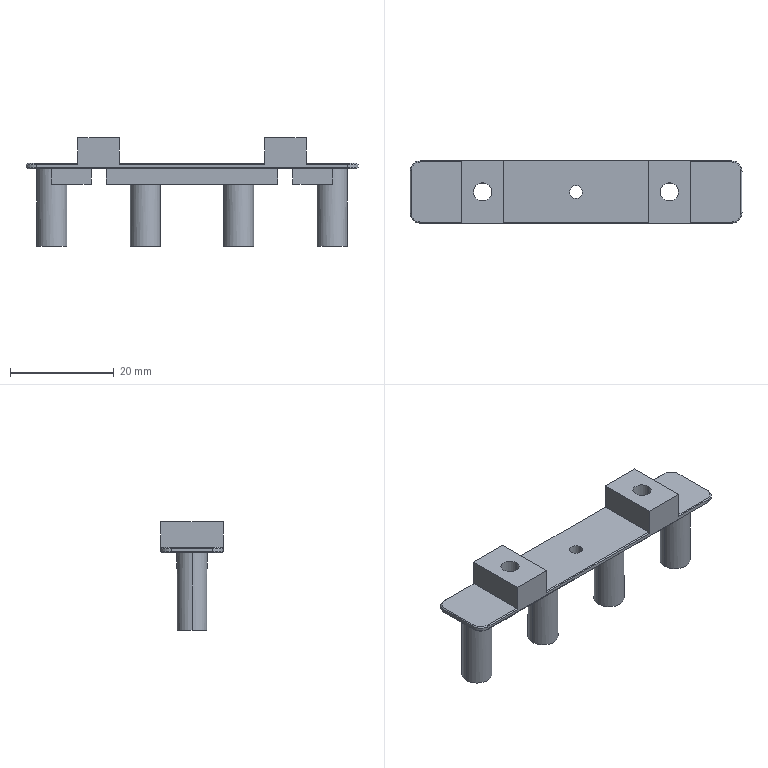NC program | NX | posted with a generic post | part box 64 x 12 x 21 mm
Lines 55 to 903 of 2110:
(ZLEVEL_PROFILE , TOOL : D10)
N90 T15 M6
N92 G54
N94 G17 G0 G90 X-37.1 Y-2.527 S9500 M3
N96 G43 Z30. H15
N98 Z1.5
N100 G94 G1 Y4.653 Z1.124 F1000.
N102 X-36.761 Y6.263 Z1.037
N104 X-36.063 Y7.752 Z0.951
N106 X-35.042 Y9.042 Z0.865
N108 X-33.752 Y10.063 Z0.779
N110 X-32.263 Y10.761 Z0.693
N112 X-30.653 Y11.1 Z0.606
N114 X0. Z-1.
N116 X30. F3000.
N118 G2 X37.1 Y4. R7.1
N120 G1 Y-4.
N122 G2 X30. Y-11.1 R7.1
N124 G1 X-30.
N126 G2 X-37.1 Y-4. R7.1
N128 G1 Y4.
N130 G2 X-30. Y11.1 R7.1
N132 G1 X0.
N134 X30. Z-1.166
N136 X30.619 Y11.073 Z-1.17
N138 X31.233 Y10.992 Z-1.173
N140 X31.838 Y10.858 Z-1.176
N142 X32.428 Y10.672 Z-1.18
N144 X33.001 Y10.435 Z-1.183
N146 X33.55 Y10.149 Z-1.187
N148 X34.072 Y9.816 Z-1.19
N150 X34.564 Y9.439 Z-1.194
N152 X35.02 Y9.02 Z-1.197
N154 X35.439 Y8.564 Z-1.2
N156 X35.816 Y8.072 Z-1.204
N158 X36.149 Y7.55 Z-1.207
N160 X36.435 Y7.001 Z-1.211
N162 X36.672 Y6.428 Z-1.214
N164 X36.858 Y5.838 Z-1.218
N166 X36.992 Y5.233 Z-1.221
N168 X37.073 Y4.619 Z-1.224
N170 X37.1 Y4. Z-1.228
N172 Y-4. Z-1.272
N174 X37.073 Y-4.619 Z-1.276
N176 X36.992 Y-5.233 Z-1.279
N178 X36.858 Y-5.838 Z-1.282
N180 X36.672 Y-6.428 Z-1.286
N182 X36.435 Y-7.001 Z-1.289
N184 X36.149 Y-7.55 Z-1.293
N186 X35.816 Y-8.072 Z-1.296
N188 X35.439 Y-8.564 Z-1.3
N190 X35.02 Y-9.02 Z-1.303
N192 X34.564 Y-9.439 Z-1.306
N194 X34.072 Y-9.816 Z-1.31
N196 X33.55 Y-10.149 Z-1.313
N198 X33.001 Y-10.435 Z-1.317
N200 X32.428 Y-10.672 Z-1.32
N202 X31.838 Y-10.858 Z-1.324
N204 X31.233 Y-10.992 Z-1.327
N206 X30.619 Y-11.073 Z-1.33
N208 X30. Y-11.1 Z-1.334
N210 X-30. Z-1.666
N212 X-30.619 Y-11.073 Z-1.67
N214 X-31.233 Y-10.992 Z-1.673
N216 X-31.838 Y-10.858 Z-1.676
N218 X-32.428 Y-10.672 Z-1.68
N220 X-33.001 Y-10.435 Z-1.683
N222 X-33.55 Y-10.149 Z-1.687
N224 X-34.072 Y-9.816 Z-1.69
N226 X-34.564 Y-9.439 Z-1.694
N228 X-35.02 Y-9.02 Z-1.697
N230 X-35.439 Y-8.564 Z-1.7
N232 X-35.816 Y-8.072 Z-1.704
N234 X-36.149 Y-7.55 Z-1.707
N236 X-36.435 Y-7.001 Z-1.711
N238 X-36.672 Y-6.428 Z-1.714
N240 X-36.858 Y-5.838 Z-1.718
N242 X-36.992 Y-5.233 Z-1.721
N244 X-37.073 Y-4.619 Z-1.724
N246 X-37.1 Y-4. Z-1.728
N248 Y4. Z-1.772
N250 X-37.073 Y4.619 Z-1.776
N252 X-36.992 Y5.233 Z-1.779
N254 X-36.858 Y5.838 Z-1.782
N256 X-36.672 Y6.428 Z-1.786
N258 X-36.435 Y7.001 Z-1.789
N260 X-36.149 Y7.55 Z-1.793
N262 X-35.816 Y8.072 Z-1.796
N264 X-35.439 Y8.564 Z-1.8
N266 X-35.02 Y9.02 Z-1.803
N268 X-34.564 Y9.439 Z-1.806
N270 X-34.072 Y9.816 Z-1.81
N272 X-33.55 Y10.149 Z-1.813
N274 X-33.001 Y10.435 Z-1.817
N276 X-32.428 Y10.672 Z-1.82
N278 X-31.838 Y10.858 Z-1.824
N280 X-31.233 Y10.992 Z-1.827
N282 X-30.619 Y11.073 Z-1.83
N284 X-30. Y11.1 Z-1.834
N286 X0. Z-2.
N288 X30. Z-2.166
N290 X30.619 Y11.073 Z-2.17
N292 X31.233 Y10.992 Z-2.173
N294 X31.838 Y10.858 Z-2.176
N296 X32.428 Y10.672 Z-2.18
N298 X33.001 Y10.435 Z-2.183
N300 X33.55 Y10.149 Z-2.187
N302 X34.072 Y9.816 Z-2.19
N304 X34.564 Y9.439 Z-2.194
N306 X35.02 Y9.02 Z-2.197
N308 X35.439 Y8.564 Z-2.2
N310 X35.816 Y8.072 Z-2.204
N312 X36.149 Y7.55 Z-2.207
N314 X36.435 Y7.001 Z-2.211
N316 X36.672 Y6.428 Z-2.214
N318 X36.858 Y5.838 Z-2.218
N320 X36.992 Y5.233 Z-2.221
N322 X37.073 Y4.619 Z-2.224
N324 X37.1 Y4. Z-2.228
N326 Y-4. Z-2.272
N328 X37.073 Y-4.619 Z-2.276
N330 X36.992 Y-5.233 Z-2.279
N332 X36.858 Y-5.838 Z-2.282
N334 X36.672 Y-6.428 Z-2.286
N336 X36.435 Y-7.001 Z-2.289
N338 X36.149 Y-7.55 Z-2.293
N340 X35.816 Y-8.072 Z-2.296
N342 X35.439 Y-8.564 Z-2.3
N344 X35.02 Y-9.02 Z-2.303
N346 X34.564 Y-9.439 Z-2.306
N348 X34.072 Y-9.816 Z-2.31
N350 X33.55 Y-10.149 Z-2.313
N352 X33.001 Y-10.435 Z-2.317
N354 X32.428 Y-10.672 Z-2.32
N356 X31.838 Y-10.858 Z-2.324
N358 X31.233 Y-10.992 Z-2.327
N360 X30.619 Y-11.073 Z-2.33
N362 X30. Y-11.1 Z-2.334
N364 X-30. Z-2.666
N366 X-30.619 Y-11.073 Z-2.67
N368 X-31.233 Y-10.992 Z-2.673
N370 X-31.838 Y-10.858 Z-2.676
N372 X-32.428 Y-10.672 Z-2.68
N374 X-33.001 Y-10.435 Z-2.683
N376 X-33.55 Y-10.149 Z-2.687
N378 X-34.072 Y-9.816 Z-2.69
N380 X-34.564 Y-9.439 Z-2.694
N382 X-35.02 Y-9.02 Z-2.697
N384 X-35.439 Y-8.564 Z-2.7
N386 X-35.816 Y-8.072 Z-2.704
N388 X-36.149 Y-7.55 Z-2.707
N390 X-36.435 Y-7.001 Z-2.711
N392 X-36.672 Y-6.428 Z-2.714
N394 X-36.858 Y-5.838 Z-2.718
N396 X-36.992 Y-5.233 Z-2.721
N398 X-37.073 Y-4.619 Z-2.724
N400 X-37.1 Y-4. Z-2.728
N402 Y4. Z-2.772
N404 X-37.073 Y4.619 Z-2.776
N406 X-36.992 Y5.233 Z-2.779
N408 X-36.858 Y5.838 Z-2.782
N410 X-36.672 Y6.428 Z-2.786
N412 X-36.435 Y7.001 Z-2.789
N414 X-36.149 Y7.55 Z-2.793
N416 X-35.816 Y8.072 Z-2.796
N418 X-35.439 Y8.564 Z-2.8
N420 X-35.02 Y9.02 Z-2.803
N422 X-34.564 Y9.439 Z-2.806
N424 X-34.072 Y9.816 Z-2.81
N426 X-33.55 Y10.149 Z-2.813
N428 X-33.001 Y10.435 Z-2.817
N430 X-32.428 Y10.672 Z-2.82
N432 X-31.838 Y10.858 Z-2.824
N434 X-31.233 Y10.992 Z-2.827
N436 X-30.619 Y11.073 Z-2.83
N438 X-30. Y11.1 Z-2.834
N440 X0. Z-3.
N442 X30. Z-3.166
N444 X30.619 Y11.073 Z-3.17
N446 X31.233 Y10.992 Z-3.173
N448 X31.838 Y10.858 Z-3.176
N450 X32.428 Y10.672 Z-3.18
N452 X33.001 Y10.435 Z-3.183
N454 X33.55 Y10.149 Z-3.187
N456 X34.072 Y9.816 Z-3.19
N458 X34.564 Y9.439 Z-3.194
N460 X35.02 Y9.02 Z-3.197
N462 X35.439 Y8.564 Z-3.2
N464 X35.816 Y8.072 Z-3.204
N466 X36.149 Y7.55 Z-3.207
N468 X36.435 Y7.001 Z-3.211
N470 X36.672 Y6.428 Z-3.214
N472 X36.858 Y5.838 Z-3.218
N474 X36.992 Y5.233 Z-3.221
N476 X37.073 Y4.619 Z-3.224
N478 X37.1 Y4. Z-3.228
N480 Y-4. Z-3.272
N482 X37.073 Y-4.619 Z-3.276
N484 X36.992 Y-5.233 Z-3.279
N486 X36.858 Y-5.838 Z-3.282
N488 X36.672 Y-6.428 Z-3.286
N490 X36.435 Y-7.001 Z-3.289
N492 X36.149 Y-7.55 Z-3.293
N494 X35.816 Y-8.072 Z-3.296
N496 X35.439 Y-8.564 Z-3.3
N498 X35.02 Y-9.02 Z-3.303
N500 X34.564 Y-9.439 Z-3.306
N502 X34.072 Y-9.816 Z-3.31
N504 X33.55 Y-10.149 Z-3.313
N506 X33.001 Y-10.435 Z-3.317
N508 X32.428 Y-10.672 Z-3.32
N510 X31.838 Y-10.858 Z-3.324
N512 X31.233 Y-10.992 Z-3.327
N514 X30.619 Y-11.073 Z-3.33
N516 X30. Y-11.1 Z-3.334
N518 X-30. Z-3.666
N520 X-30.619 Y-11.073 Z-3.67
N522 X-31.233 Y-10.992 Z-3.673
N524 X-31.838 Y-10.858 Z-3.676
N526 X-32.428 Y-10.672 Z-3.68
N528 X-33.001 Y-10.435 Z-3.683
N530 X-33.55 Y-10.149 Z-3.687
N532 X-34.072 Y-9.816 Z-3.69
N534 X-34.564 Y-9.439 Z-3.694
N536 X-35.02 Y-9.02 Z-3.697
N538 X-35.439 Y-8.564 Z-3.7
N540 X-35.816 Y-8.072 Z-3.704
N542 X-36.149 Y-7.55 Z-3.707
N544 X-36.435 Y-7.001 Z-3.711
N546 X-36.672 Y-6.428 Z-3.714
N548 X-36.858 Y-5.838 Z-3.718
N550 X-36.992 Y-5.233 Z-3.721
N552 X-37.073 Y-4.619 Z-3.724
N554 X-37.1 Y-4. Z-3.728
N556 Y4. Z-3.772
N558 X-37.073 Y4.619 Z-3.776
N560 X-36.992 Y5.233 Z-3.779
N562 X-36.858 Y5.838 Z-3.782
N564 X-36.672 Y6.428 Z-3.786
N566 X-36.435 Y7.001 Z-3.789
N568 X-36.149 Y7.55 Z-3.793
N570 X-35.816 Y8.072 Z-3.796
N572 X-35.439 Y8.564 Z-3.8
N574 X-35.02 Y9.02 Z-3.803
N576 X-34.564 Y9.439 Z-3.806
N578 X-34.072 Y9.816 Z-3.81
N580 X-33.55 Y10.149 Z-3.813
N582 X-33.001 Y10.435 Z-3.817
N584 X-32.428 Y10.672 Z-3.82
N586 X-31.838 Y10.858 Z-3.824
N588 X-31.233 Y10.992 Z-3.827
N590 X-30.619 Y11.073 Z-3.83
N592 X-30. Y11.1 Z-3.834
N594 X0. Z-4.
N596 X30. Z-4.166
N598 X30.619 Y11.073 Z-4.17
N600 X31.233 Y10.992 Z-4.173
N602 X31.838 Y10.858 Z-4.176
N604 X32.428 Y10.672 Z-4.18
N606 X33.001 Y10.435 Z-4.183
N608 X33.55 Y10.149 Z-4.187
N610 X34.072 Y9.816 Z-4.19
N612 X34.564 Y9.439 Z-4.194
N614 X35.02 Y9.02 Z-4.197
N616 X35.439 Y8.564 Z-4.2
N618 X35.816 Y8.072 Z-4.204
N620 X36.149 Y7.55 Z-4.207
N622 X36.435 Y7.001 Z-4.211
N624 X36.672 Y6.428 Z-4.214
N626 X36.858 Y5.838 Z-4.218
N628 X36.992 Y5.233 Z-4.221
N630 X37.073 Y4.619 Z-4.224
N632 X37.1 Y4. Z-4.228
N634 Y-4. Z-4.272
N636 X37.073 Y-4.619 Z-4.276
N638 X36.992 Y-5.233 Z-4.279
N640 X36.858 Y-5.838 Z-4.282
N642 X36.672 Y-6.428 Z-4.286
N644 X36.435 Y-7.001 Z-4.289
N646 X36.149 Y-7.55 Z-4.293
N648 X35.816 Y-8.072 Z-4.296
N650 X35.439 Y-8.564 Z-4.3
N652 X35.02 Y-9.02 Z-4.303
N654 X34.564 Y-9.439 Z-4.306
N656 X34.072 Y-9.816 Z-4.31
N658 X33.55 Y-10.149 Z-4.313
N660 X33.001 Y-10.435 Z-4.317
N662 X32.428 Y-10.672 Z-4.32
N664 X31.838 Y-10.858 Z-4.324
N666 X31.233 Y-10.992 Z-4.327
N668 X30.619 Y-11.073 Z-4.33
N670 X30. Y-11.1 Z-4.334
N672 X-30. Z-4.666
N674 X-30.619 Y-11.073 Z-4.67
N676 X-31.233 Y-10.992 Z-4.673
N678 X-31.838 Y-10.858 Z-4.676
N680 X-32.428 Y-10.672 Z-4.68
N682 X-33.001 Y-10.435 Z-4.683
N684 X-33.55 Y-10.149 Z-4.687
N686 X-34.072 Y-9.816 Z-4.69
N688 X-34.564 Y-9.439 Z-4.694
N690 X-35.02 Y-9.02 Z-4.697
N692 X-35.439 Y-8.564 Z-4.7
N694 X-35.816 Y-8.072 Z-4.704
N696 X-36.149 Y-7.55 Z-4.707
N698 X-36.435 Y-7.001 Z-4.711
N700 X-36.672 Y-6.428 Z-4.714
N702 X-36.858 Y-5.838 Z-4.718
N704 X-36.992 Y-5.233 Z-4.721
N706 X-37.073 Y-4.619 Z-4.724
N708 X-37.1 Y-4. Z-4.728
N710 Y4. Z-4.772
N712 X-37.073 Y4.619 Z-4.776
N714 X-36.992 Y5.233 Z-4.779
N716 X-36.858 Y5.838 Z-4.782
N718 X-36.672 Y6.428 Z-4.786
N720 X-36.435 Y7.001 Z-4.789
N722 X-36.149 Y7.55 Z-4.793
N724 X-35.816 Y8.072 Z-4.796
N726 X-35.439 Y8.564 Z-4.8
N728 X-35.02 Y9.02 Z-4.803
N730 X-34.564 Y9.439 Z-4.806
N732 X-34.072 Y9.816 Z-4.81
N734 X-33.55 Y10.149 Z-4.813
N736 X-33.001 Y10.435 Z-4.817
N738 X-32.428 Y10.672 Z-4.82
N740 X-31.838 Y10.858 Z-4.824
N742 X-31.233 Y10.992 Z-4.827
N744 X-30.619 Y11.073 Z-4.83
N746 X-30. Y11.1 Z-4.834
N748 X0. Z-5.
N750 X30. Z-5.166
N752 X30.619 Y11.073 Z-5.17
N754 X31.233 Y10.992 Z-5.173
N756 X31.838 Y10.858 Z-5.176
N758 X32.428 Y10.672 Z-5.18
N760 X33.001 Y10.435 Z-5.183
N762 X33.55 Y10.149 Z-5.187
N764 X34.072 Y9.816 Z-5.19
N766 X34.564 Y9.439 Z-5.194
N768 X35.02 Y9.02 Z-5.197
N770 X35.439 Y8.564 Z-5.2
N772 X35.816 Y8.072 Z-5.204
N774 X36.149 Y7.55 Z-5.207
N776 X36.435 Y7.001 Z-5.211
N778 X36.672 Y6.428 Z-5.214
N780 X36.858 Y5.838 Z-5.218
N782 X36.992 Y5.233 Z-5.221
N784 X37.073 Y4.619 Z-5.224
N786 X37.1 Y4. Z-5.228
N788 Y-4. Z-5.272
N790 X37.073 Y-4.619 Z-5.276
N792 X36.992 Y-5.233 Z-5.279
N794 X36.858 Y-5.838 Z-5.282
N796 X36.672 Y-6.428 Z-5.286
N798 X36.435 Y-7.001 Z-5.289
N800 X36.149 Y-7.55 Z-5.293
N802 X35.816 Y-8.072 Z-5.296
N804 X35.439 Y-8.564 Z-5.3
N806 X35.02 Y-9.02 Z-5.303
N808 X34.564 Y-9.439 Z-5.306
N810 X34.072 Y-9.816 Z-5.31
N812 X33.55 Y-10.149 Z-5.313
N814 X33.001 Y-10.435 Z-5.317
N816 X32.428 Y-10.672 Z-5.32
N818 X31.838 Y-10.858 Z-5.324
N820 X31.233 Y-10.992 Z-5.327
N822 X30.619 Y-11.073 Z-5.33
N824 X30. Y-11.1 Z-5.334
N826 X-30. Z-5.666
N828 X-30.619 Y-11.073 Z-5.67
N830 X-31.233 Y-10.992 Z-5.673
N832 X-31.838 Y-10.858 Z-5.676
N834 X-32.428 Y-10.672 Z-5.68
N836 X-33.001 Y-10.435 Z-5.683
N838 X-33.55 Y-10.149 Z-5.687
N840 X-34.072 Y-9.816 Z-5.69
N842 X-34.564 Y-9.439 Z-5.694
N844 X-35.02 Y-9.02 Z-5.697
N846 X-35.439 Y-8.564 Z-5.7
N848 X-35.816 Y-8.072 Z-5.704
N850 X-36.149 Y-7.55 Z-5.707
N852 X-36.435 Y-7.001 Z-5.711
N854 X-36.672 Y-6.428 Z-5.714
N856 X-36.858 Y-5.838 Z-5.718
N858 X-36.992 Y-5.233 Z-5.721
N860 X-37.073 Y-4.619 Z-5.724
N862 X-37.1 Y-4. Z-5.728
N864 Y4. Z-5.772
N866 X-37.073 Y4.619 Z-5.776
N868 X-36.992 Y5.233 Z-5.779
N870 X-36.858 Y5.838 Z-5.782
N872 X-36.672 Y6.428 Z-5.786
N874 X-36.435 Y7.001 Z-5.789
N876 X-36.149 Y7.55 Z-5.793
N878 X-35.816 Y8.072 Z-5.796
N880 X-35.439 Y8.564 Z-5.8
N882 X-35.02 Y9.02 Z-5.803
N884 X-34.564 Y9.439 Z-5.806
N886 X-34.072 Y9.816 Z-5.81
N888 X-33.55 Y10.149 Z-5.813
N890 X-33.001 Y10.435 Z-5.817
N892 X-32.428 Y10.672 Z-5.82
N894 X-31.838 Y10.858 Z-5.824
N896 X-31.233 Y10.992 Z-5.827
N898 X-30.619 Y11.073 Z-5.83
N900 X-30. Y11.1 Z-5.834
N902 X0. Z-6.
N904 X30. Z-6.166
N906 X30.619 Y11.073 Z-6.17
N908 X31.233 Y10.992 Z-6.173
N910 X31.838 Y10.858 Z-6.176
N912 X32.428 Y10.672 Z-6.18
N914 X33.001 Y10.435 Z-6.183
N916 X33.55 Y10.149 Z-6.187
N918 X34.072 Y9.816 Z-6.19
N920 X34.564 Y9.439 Z-6.194
N922 X35.02 Y9.02 Z-6.197
N924 X35.439 Y8.564 Z-6.2
N926 X35.816 Y8.072 Z-6.204
N928 X36.149 Y7.55 Z-6.207
N930 X36.435 Y7.001 Z-6.211
N932 X36.672 Y6.428 Z-6.214
N934 X36.858 Y5.838 Z-6.218
N936 X36.992 Y5.233 Z-6.221
N938 X37.073 Y4.619 Z-6.224
N940 X37.1 Y4. Z-6.228
N942 Y-4. Z-6.272
N944 X37.073 Y-4.619 Z-6.276
N946 X36.992 Y-5.233 Z-6.279
N948 X36.858 Y-5.838 Z-6.282
N950 X36.672 Y-6.428 Z-6.286
N952 X36.435 Y-7.001 Z-6.289
N954 X36.149 Y-7.55 Z-6.293
N956 X35.816 Y-8.072 Z-6.296
N958 X35.439 Y-8.564 Z-6.3
N960 X35.02 Y-9.02 Z-6.303
N962 X34.564 Y-9.439 Z-6.306
N964 X34.072 Y-9.816 Z-6.31
N966 X33.55 Y-10.149 Z-6.313
N968 X33.001 Y-10.435 Z-6.317
N970 X32.428 Y-10.672 Z-6.32
N972 X31.838 Y-10.858 Z-6.324
N974 X31.233 Y-10.992 Z-6.327
N976 X30.619 Y-11.073 Z-6.33
N978 X30. Y-11.1 Z-6.334
N980 X-30. Z-6.666
N982 X-30.619 Y-11.073 Z-6.67
N984 X-31.233 Y-10.992 Z-6.673
N986 X-31.838 Y-10.858 Z-6.676
N988 X-32.428 Y-10.672 Z-6.68
N990 X-33.001 Y-10.435 Z-6.683
N992 X-33.55 Y-10.149 Z-6.687
N994 X-34.072 Y-9.816 Z-6.69
N996 X-34.564 Y-9.439 Z-6.694
N998 X-35.02 Y-9.02 Z-6.697
N1000 X-35.439 Y-8.564 Z-6.7
N1002 X-35.816 Y-8.072 Z-6.704
N1004 X-36.149 Y-7.55 Z-6.707
N1006 X-36.435 Y-7.001 Z-6.711
N1008 X-36.672 Y-6.428 Z-6.714
N1010 X-36.858 Y-5.838 Z-6.718
N1012 X-36.992 Y-5.233 Z-6.721
N1014 X-37.073 Y-4.619 Z-6.724
N1016 X-37.1 Y-4. Z-6.728
N1018 Y4. Z-6.772
N1020 X-37.073 Y4.619 Z-6.776
N1022 X-36.992 Y5.233 Z-6.779
N1024 X-36.858 Y5.838 Z-6.782
N1026 X-36.672 Y6.428 Z-6.786
N1028 X-36.435 Y7.001 Z-6.789
N1030 X-36.149 Y7.55 Z-6.793
N1032 X-35.816 Y8.072 Z-6.796
N1034 X-35.439 Y8.564 Z-6.8
N1036 X-35.02 Y9.02 Z-6.803
N1038 X-34.564 Y9.439 Z-6.806
N1040 X-34.072 Y9.816 Z-6.81
N1042 X-33.55 Y10.149 Z-6.813
N1044 X-33.001 Y10.435 Z-6.817
N1046 X-32.428 Y10.672 Z-6.82
N1048 X-31.838 Y10.858 Z-6.824
N1050 X-31.233 Y10.992 Z-6.827
N1052 X-30.619 Y11.073 Z-6.83
N1054 X-30. Y11.1 Z-6.834
N1056 X0. Z-7.
N1058 X30. Z-7.166
N1060 X30.619 Y11.073 Z-7.17
N1062 X31.233 Y10.992 Z-7.173
N1064 X31.838 Y10.858 Z-7.176
N1066 X32.428 Y10.672 Z-7.18
N1068 X33.001 Y10.435 Z-7.183
N1070 X33.55 Y10.149 Z-7.187
N1072 X34.072 Y9.816 Z-7.19
N1074 X34.564 Y9.439 Z-7.194
N1076 X35.02 Y9.02 Z-7.197
N1078 X35.439 Y8.564 Z-7.2
N1080 X35.816 Y8.072 Z-7.204
N1082 X36.149 Y7.55 Z-7.207
N1084 X36.435 Y7.001 Z-7.211
N1086 X36.672 Y6.428 Z-7.214
N1088 X36.858 Y5.838 Z-7.218
N1090 X36.992 Y5.233 Z-7.221
N1092 X37.073 Y4.619 Z-7.224
N1094 X37.1 Y4. Z-7.228
N1096 Y-4. Z-7.272
N1098 X37.073 Y-4.619 Z-7.276
N1100 X36.992 Y-5.233 Z-7.279
N1102 X36.858 Y-5.838 Z-7.282
N1104 X36.672 Y-6.428 Z-7.286
N1106 X36.435 Y-7.001 Z-7.289
N1108 X36.149 Y-7.55 Z-7.293
N1110 X35.816 Y-8.072 Z-7.296
N1112 X35.439 Y-8.564 Z-7.3
N1114 X35.02 Y-9.02 Z-7.303
N1116 X34.564 Y-9.439 Z-7.306
N1118 X34.072 Y-9.816 Z-7.31
N1120 X33.55 Y-10.149 Z-7.313
N1122 X33.001 Y-10.435 Z-7.317
N1124 X32.428 Y-10.672 Z-7.32
N1126 X31.838 Y-10.858 Z-7.324
N1128 X31.233 Y-10.992 Z-7.327
N1130 X30.619 Y-11.073 Z-7.33
N1132 X30. Y-11.1 Z-7.334
N1134 X-30. Z-7.666
N1136 X-30.619 Y-11.073 Z-7.67
N1138 X-31.233 Y-10.992 Z-7.673
N1140 X-31.838 Y-10.858 Z-7.676
N1142 X-32.428 Y-10.672 Z-7.68
N1144 X-33.001 Y-10.435 Z-7.683
N1146 X-33.55 Y-10.149 Z-7.687
N1148 X-34.072 Y-9.816 Z-7.69
N1150 X-34.564 Y-9.439 Z-7.694
N1152 X-35.02 Y-9.02 Z-7.697
N1154 X-35.439 Y-8.564 Z-7.7
N1156 X-35.816 Y-8.072 Z-7.704
N1158 X-36.149 Y-7.55 Z-7.707
N1160 X-36.435 Y-7.001 Z-7.711
N1162 X-36.672 Y-6.428 Z-7.714
N1164 X-36.858 Y-5.838 Z-7.718
N1166 X-36.992 Y-5.233 Z-7.721
N1168 X-37.073 Y-4.619 Z-7.724
N1170 X-37.1 Y-4. Z-7.728
N1172 Y4. Z-7.772
N1174 X-37.073 Y4.619 Z-7.776
N1176 X-36.992 Y5.233 Z-7.779
N1178 X-36.858 Y5.838 Z-7.782
N1180 X-36.672 Y6.428 Z-7.786
N1182 X-36.435 Y7.001 Z-7.789
N1184 X-36.149 Y7.55 Z-7.793
N1186 X-35.816 Y8.072 Z-7.796
N1188 X-35.439 Y8.564 Z-7.8
N1190 X-35.02 Y9.02 Z-7.803
N1192 X-34.564 Y9.439 Z-7.806
N1194 X-34.072 Y9.816 Z-7.81
N1196 X-33.55 Y10.149 Z-7.813
N1198 X-33.001 Y10.435 Z-7.817
N1200 X-32.428 Y10.672 Z-7.82
N1202 X-31.838 Y10.858 Z-7.824
N1204 X-31.233 Y10.992 Z-7.827
N1206 X-30.619 Y11.073 Z-7.83
N1208 X-30. Y11.1 Z-7.834
N1210 X0. Z-8.
N1212 X30. Z-8.166
N1214 X30.619 Y11.073 Z-8.17
N1216 X31.233 Y10.992 Z-8.173
N1218 X31.838 Y10.858 Z-8.176
N1220 X32.428 Y10.672 Z-8.18
N1222 X33.001 Y10.435 Z-8.183
N1224 X33.55 Y10.149 Z-8.187
N1226 X34.072 Y9.816 Z-8.19
N1228 X34.564 Y9.439 Z-8.194
N1230 X35.02 Y9.02 Z-8.197
N1232 X35.439 Y8.564 Z-8.2
N1234 X35.816 Y8.072 Z-8.204
N1236 X36.149 Y7.55 Z-8.207
N1238 X36.435 Y7.001 Z-8.211
N1240 X36.672 Y6.428 Z-8.214
N1242 X36.858 Y5.838 Z-8.218
N1244 X36.992 Y5.233 Z-8.221
N1246 X37.073 Y4.619 Z-8.224
N1248 X37.1 Y4. Z-8.228
N1250 Y-4. Z-8.272
N1252 X37.073 Y-4.619 Z-8.276
N1254 X36.992 Y-5.233 Z-8.279
N1256 X36.858 Y-5.838 Z-8.282
N1258 X36.672 Y-6.428 Z-8.286
N1260 X36.435 Y-7.001 Z-8.289
N1262 X36.149 Y-7.55 Z-8.293
N1264 X35.816 Y-8.072 Z-8.296
N1266 X35.439 Y-8.564 Z-8.3
N1268 X35.02 Y-9.02 Z-8.303
N1270 X34.564 Y-9.439 Z-8.306
N1272 X34.072 Y-9.816 Z-8.31
N1274 X33.55 Y-10.149 Z-8.313
N1276 X33.001 Y-10.435 Z-8.317
N1278 X32.428 Y-10.672 Z-8.32
N1280 X31.838 Y-10.858 Z-8.324
N1282 X31.233 Y-10.992 Z-8.327
N1284 X30.619 Y-11.073 Z-8.33
N1286 X30. Y-11.1 Z-8.334
N1288 X-30. Z-8.666
N1290 X-30.619 Y-11.073 Z-8.67
N1292 X-31.233 Y-10.992 Z-8.673
N1294 X-31.838 Y-10.858 Z-8.676
N1296 X-32.428 Y-10.672 Z-8.68
N1298 X-33.001 Y-10.435 Z-8.683
N1300 X-33.55 Y-10.149 Z-8.687
N1302 X-34.072 Y-9.816 Z-8.69
N1304 X-34.564 Y-9.439 Z-8.694
N1306 X-35.02 Y-9.02 Z-8.697
N1308 X-35.439 Y-8.564 Z-8.7
N1310 X-35.816 Y-8.072 Z-8.704
N1312 X-36.149 Y-7.55 Z-8.707
N1314 X-36.435 Y-7.001 Z-8.711
N1316 X-36.672 Y-6.428 Z-8.714
N1318 X-36.858 Y-5.838 Z-8.718
N1320 X-36.992 Y-5.233 Z-8.721
N1322 X-37.073 Y-4.619 Z-8.724
N1324 X-37.1 Y-4. Z-8.728
N1326 Y4. Z-8.772
N1328 X-37.073 Y4.619 Z-8.776
N1330 X-36.992 Y5.233 Z-8.779
N1332 X-36.858 Y5.838 Z-8.782
N1334 X-36.672 Y6.428 Z-8.786
N1336 X-36.435 Y7.001 Z-8.789
N1338 X-36.149 Y7.55 Z-8.793
N1340 X-35.816 Y8.072 Z-8.796
N1342 X-35.439 Y8.564 Z-8.8
N1344 X-35.02 Y9.02 Z-8.803
N1346 X-34.564 Y9.439 Z-8.806
N1348 X-34.072 Y9.816 Z-8.81
N1350 X-33.55 Y10.149 Z-8.813
N1352 X-33.001 Y10.435 Z-8.817
N1354 X-32.428 Y10.672 Z-8.82
N1356 X-31.838 Y10.858 Z-8.824
N1358 X-31.233 Y10.992 Z-8.827
N1360 X-30.619 Y11.073 Z-8.83
N1362 X-30. Y11.1 Z-8.834
N1364 X0. Z-9.
N1366 X30. Z-9.166
N1368 X30.619 Y11.073 Z-9.17
N1370 X31.233 Y10.992 Z-9.173
N1372 X31.838 Y10.858 Z-9.176
N1374 X32.428 Y10.672 Z-9.18
N1376 X33.001 Y10.435 Z-9.183
N1378 X33.55 Y10.149 Z-9.187
N1380 X34.072 Y9.816 Z-9.19
N1382 X34.564 Y9.439 Z-9.194
N1384 X35.02 Y9.02 Z-9.197
N1386 X35.439 Y8.564 Z-9.2
N1388 X35.816 Y8.072 Z-9.204
N1390 X36.149 Y7.55 Z-9.207
N1392 X36.435 Y7.001 Z-9.211
N1394 X36.672 Y6.428 Z-9.214
N1396 X36.858 Y5.838 Z-9.218
N1398 X36.992 Y5.233 Z-9.221
N1400 X37.073 Y4.619 Z-9.224
N1402 X37.1 Y4. Z-9.228
N1404 Y-4. Z-9.272
N1406 X37.073 Y-4.619 Z-9.276
N1408 X36.992 Y-5.233 Z-9.279
N1410 X36.858 Y-5.838 Z-9.282
N1412 X36.672 Y-6.428 Z-9.286
N1414 X36.435 Y-7.001 Z-9.289
N1416 X36.149 Y-7.55 Z-9.293
N1418 X35.816 Y-8.072 Z-9.296
N1420 X35.439 Y-8.564 Z-9.3
N1422 X35.02 Y-9.02 Z-9.303
N1424 X34.564 Y-9.439 Z-9.306
N1426 X34.072 Y-9.816 Z-9.31
N1428 X33.55 Y-10.149 Z-9.313
N1430 X33.001 Y-10.435 Z-9.317
N1432 X32.428 Y-10.672 Z-9.32
N1434 X31.838 Y-10.858 Z-9.324
N1436 X31.233 Y-10.992 Z-9.327
N1438 X30.619 Y-11.073 Z-9.33
N1440 X30. Y-11.1 Z-9.334
N1442 X-30. Z-9.666
N1444 X-30.619 Y-11.073 Z-9.67
N1446 X-31.233 Y-10.992 Z-9.673
N1448 X-31.838 Y-10.858 Z-9.676
N1450 X-32.428 Y-10.672 Z-9.68
N1452 X-33.001 Y-10.435 Z-9.683
N1454 X-33.55 Y-10.149 Z-9.687
N1456 X-34.072 Y-9.816 Z-9.69
N1458 X-34.564 Y-9.439 Z-9.694
N1460 X-35.02 Y-9.02 Z-9.697
N1462 X-35.439 Y-8.564 Z-9.7
N1464 X-35.816 Y-8.072 Z-9.704
N1466 X-36.149 Y-7.55 Z-9.707
N1468 X-36.435 Y-7.001 Z-9.711
N1470 X-36.672 Y-6.428 Z-9.714
N1472 X-36.858 Y-5.838 Z-9.718
N1474 X-36.992 Y-5.233 Z-9.721
N1476 X-37.073 Y-4.619 Z-9.724
N1478 X-37.1 Y-4. Z-9.728
N1480 Y4. Z-9.772
N1482 X-37.073 Y4.619 Z-9.776
N1484 X-36.992 Y5.233 Z-9.779
N1486 X-36.858 Y5.838 Z-9.782
N1488 X-36.672 Y6.428 Z-9.786
N1490 X-36.435 Y7.001 Z-9.789
N1492 X-36.149 Y7.55 Z-9.793
N1494 X-35.816 Y8.072 Z-9.796
N1496 X-35.439 Y8.564 Z-9.8
N1498 X-35.02 Y9.02 Z-9.803
N1500 X-34.564 Y9.439 Z-9.806
N1502 X-34.072 Y9.816 Z-9.81
N1504 X-33.55 Y10.149 Z-9.813
N1506 X-33.001 Y10.435 Z-9.817
N1508 X-32.428 Y10.672 Z-9.82
N1510 X-31.838 Y10.858 Z-9.824
N1512 X-31.233 Y10.992 Z-9.827
N1514 X-30.619 Y11.073 Z-9.83
N1516 X-30. Y11.1 Z-9.834
N1518 X0. Z-10.
N1520 X30. Z-10.166
N1522 X30.619 Y11.073 Z-10.17
N1524 X31.233 Y10.992 Z-10.173
N1526 X31.838 Y10.858 Z-10.176
N1528 X32.428 Y10.672 Z-10.18
N1530 X33.001 Y10.435 Z-10.183
N1532 X33.55 Y10.149 Z-10.187
N1534 X34.072 Y9.816 Z-10.19
N1536 X34.564 Y9.439 Z-10.194
N1538 X35.02 Y9.02 Z-10.197
N1540 X35.439 Y8.564 Z-10.2
N1542 X35.816 Y8.072 Z-10.204
N1544 X36.149 Y7.55 Z-10.207
N1546 X36.435 Y7.001 Z-10.211
N1548 X36.672 Y6.428 Z-10.214
N1550 X36.858 Y5.838 Z-10.218
N1552 X36.992 Y5.233 Z-10.221
N1554 X37.073 Y4.619 Z-10.224
N1556 X37.1 Y4. Z-10.228
N1558 Y-4. Z-10.272
N1560 X37.073 Y-4.619 Z-10.276
N1562 X36.992 Y-5.233 Z-10.279
N1564 X36.858 Y-5.838 Z-10.282
N1566 X36.672 Y-6.428 Z-10.286
N1568 X36.435 Y-7.001 Z-10.289
N1570 X36.149 Y-7.55 Z-10.293
N1572 X35.816 Y-8.072 Z-10.296
N1574 X35.439 Y-8.564 Z-10.3
N1576 X35.02 Y-9.02 Z-10.303
N1578 X34.564 Y-9.439 Z-10.306
N1580 X34.072 Y-9.816 Z-10.31
N1582 X33.55 Y-10.149 Z-10.313
N1584 X33.001 Y-10.435 Z-10.317
N1586 X32.428 Y-10.672 Z-10.32
N1588 X31.838 Y-10.858 Z-10.324
N1590 X31.233 Y-10.992 Z-10.327
N1592 X30.619 Y-11.073 Z-10.33
N1594 X30. Y-11.1 Z-10.334
N1596 X-30. Z-10.666
N1598 X-30.619 Y-11.073 Z-10.67
N1600 X-31.233 Y-10.992 Z-10.673
N1602 X-31.838 Y-10.858 Z-10.676
N1604 X-32.428 Y-10.672 Z-10.68
N1606 X-33.001 Y-10.435 Z-10.683
N1608 X-33.55 Y-10.149 Z-10.687
N1610 X-34.072 Y-9.816 Z-10.69
N1612 X-34.564 Y-9.439 Z-10.694
N1614 X-35.02 Y-9.02 Z-10.697
N1616 X-35.439 Y-8.564 Z-10.7
N1618 X-35.816 Y-8.072 Z-10.704
N1620 X-36.149 Y-7.55 Z-10.707
N1622 X-36.435 Y-7.001 Z-10.711
N1624 X-36.672 Y-6.428 Z-10.714
N1626 X-36.858 Y-5.838 Z-10.718
N1628 X-36.992 Y-5.233 Z-10.721
N1630 X-37.073 Y-4.619 Z-10.724
N1632 X-37.1 Y-4. Z-10.728
N1634 Y4. Z-10.772
N1636 X-37.073 Y4.619 Z-10.776
N1638 X-36.992 Y5.233 Z-10.779
N1640 X-36.858 Y5.838 Z-10.782
N1642 X-36.672 Y6.428 Z-10.786
N1644 X-36.435 Y7.001 Z-10.789
N1646 X-36.149 Y7.55 Z-10.793
N1648 X-35.816 Y8.072 Z-10.796
N1650 X-35.439 Y8.564 Z-10.8
N1652 X-35.02 Y9.02 Z-10.803
N1654 X-34.564 Y9.439 Z-10.806
N1656 X-34.072 Y9.816 Z-10.81
N1658 X-33.55 Y10.149 Z-10.813
N1660 X-33.001 Y10.435 Z-10.817
N1662 X-32.428 Y10.672 Z-10.82
N1664 X-31.838 Y10.858 Z-10.824
N1666 X-31.233 Y10.992 Z-10.827
N1668 X-30.619 Y11.073 Z-10.83
N1670 X-30. Y11.1 Z-10.834
N1672 X0. Z-11.
N1674 X30. Z-11.166
N1676 X30.619 Y11.073 Z-11.17
N1678 X31.233 Y10.992 Z-11.173
N1680 X31.838 Y10.858 Z-11.176
N1682 X32.428 Y10.672 Z-11.18
N1684 X33.001 Y10.435 Z-11.183
N1686 X33.55 Y10.149 Z-11.187
N1688 X34.072 Y9.816 Z-11.19
N1690 X34.564 Y9.439 Z-11.194
N1692 X35.02 Y9.02 Z-11.197
N1694 X35.439 Y8.564 Z-11.2
N1696 X35.816 Y8.072 Z-11.204
N1698 X36.149 Y7.55 Z-11.207
N1700 X36.435 Y7.001 Z-11.211
N1702 X36.672 Y6.428 Z-11.214
N1704 X36.858 Y5.838 Z-11.218
N1706 X36.992 Y5.233 Z-11.221
N1708 X37.073 Y4.619 Z-11.224
N1710 X37.1 Y4. Z-11.228
N1712 Y-4. Z-11.272
N1714 X37.073 Y-4.619 Z-11.276
N1716 X36.992 Y-5.233 Z-11.279
N1718 X36.858 Y-5.838 Z-11.282
N1720 X36.672 Y-6.428 Z-11.286
N1722 X36.435 Y-7.001 Z-11.289
N1724 X36.149 Y-7.55 Z-11.293
N1726 X35.816 Y-8.072 Z-11.296
N1728 X35.439 Y-8.564 Z-11.3
N1730 X35.02 Y-9.02 Z-11.303
N1732 X34.564 Y-9.439 Z-11.306
N1734 X34.072 Y-9.816 Z-11.31
N1736 X33.55 Y-10.149 Z-11.313
N1738 X33.001 Y-10.435 Z-11.317
N1740 X32.428 Y-10.672 Z-11.32
N1742 X31.838 Y-10.858 Z-11.324
N1744 X31.233 Y-10.992 Z-11.327
N1746 X30.619 Y-11.073 Z-11.33
N1748 X30. Y-11.1 Z-11.334
N1750 X-30. Z-11.666
N1752 X-30.619 Y-11.073 Z-11.67
N1754 X-31.233 Y-10.992 Z-11.673
N1756 X-31.838 Y-10.858 Z-11.676
N1758 X-32.428 Y-10.672 Z-11.68
N1760 X-33.001 Y-10.435 Z-11.683
N1762 X-33.55 Y-10.149 Z-11.687
N1764 X-34.072 Y-9.816 Z-11.69
N1766 X-34.564 Y-9.439 Z-11.694
N1768 X-35.02 Y-9.02 Z-11.697
N1770 X-35.439 Y-8.564 Z-11.7
N1772 X-35.816 Y-8.072 Z-11.704
N1774 X-36.149 Y-7.55 Z-11.707
N1776 X-36.435 Y-7.001 Z-11.711
N1778 X-36.672 Y-6.428 Z-11.714
N1780 X-36.858 Y-5.838 Z-11.718